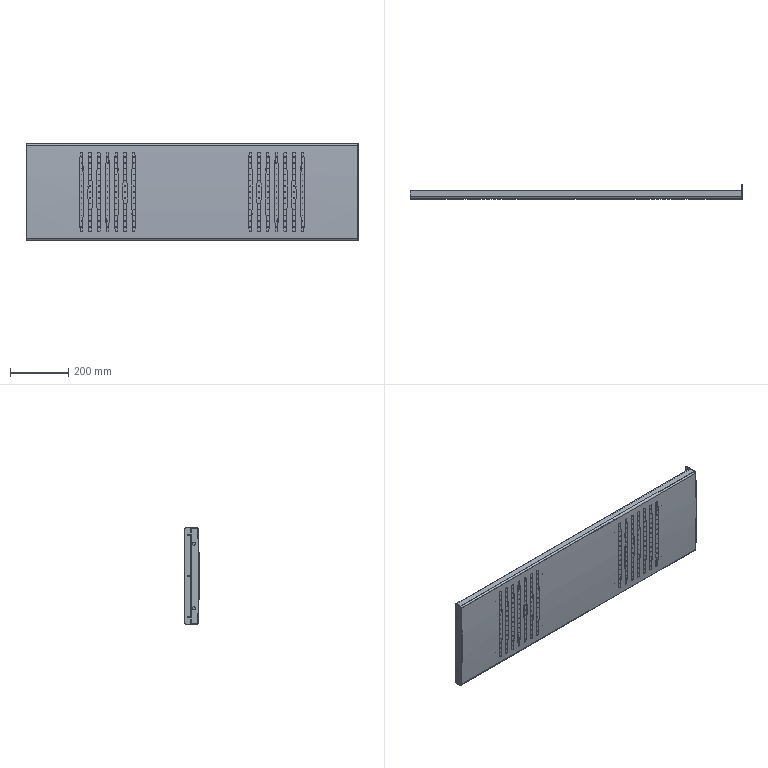Part | STEP file | 1519D3-1_AF0.stp.STEP | 4 solids | 593 faces | box 1140 x 50 x 332 mm | volume 997940 mm3 | cylinder 389 | spline 98 | plane 90 | cone 16 | commonest cylinder face diameters 2 x364 5 x6 12.4 x6 10.5 x4 7832 x3 8.4 x2